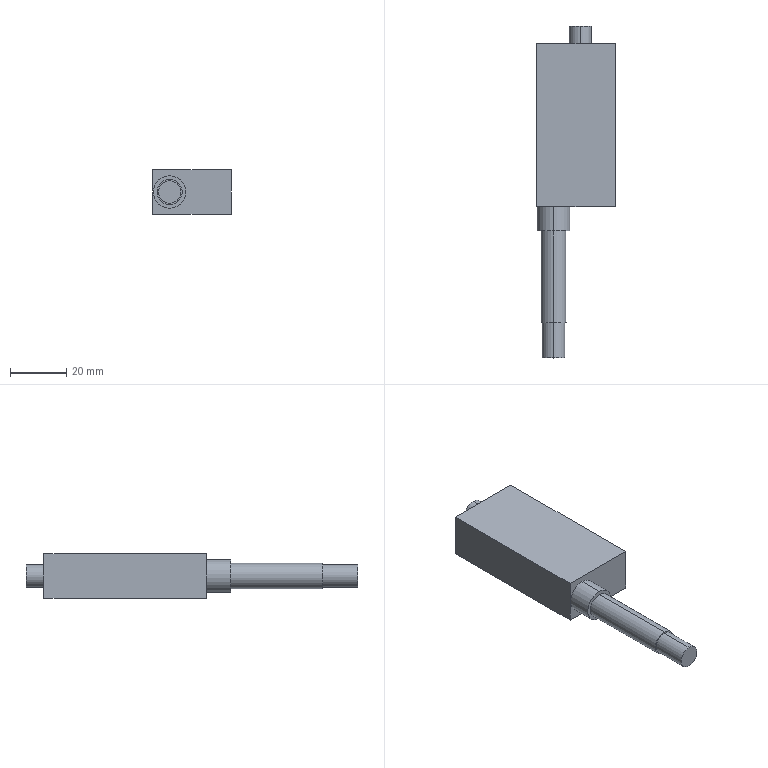Part | STEP file | Sensor head GT2-H12 | 1 solid | 18 faces | box 28 x 118.4 x 16 mm | volume 29940 mm3 | plane 10 | cylinder 8 | commonest cylinder face diameters 8 x4 9 x2 11.6 x2
STEP:
#1=CARTESIAN_POINT('',(0.,0.,0.));
#2=DIRECTION('',(0.,0.,1.));
#3=DIRECTION('',(1.,0.,0.));
#4=AXIS2_PLACEMENT_3D('',#1,#2,#3);
#5=CARTESIAN_POINT('',(-8.,-37.7,5.8));
#6=VERTEX_POINT('',#5);
#7=CARTESIAN_POINT('',(-8.,-37.7,-5.8));
#8=VERTEX_POINT('',#7);
#9=CARTESIAN_POINT('',(-8.,-37.7,0.));
#10=DIRECTION('',(0.,1.,0.));
#11=DIRECTION('',(0.,0.,1.));
#12=AXIS2_PLACEMENT_3D('',#9,#10,#11);
#13=CIRCLE('',#12,5.8);
#14=CARTESIAN_POINT('',(-8.,-37.7,0.));
#15=DIRECTION('',(0.,1.,0.));
#16=DIRECTION('',(0.,0.,1.));
#17=AXIS2_PLACEMENT_3D('',#14,#15,#16);
#18=CYLINDRICAL_SURFACE('',#17,5.8);
#19=CARTESIAN_POINT('',(0.,0.));
#20=DIRECTION('',(1.,0.));
#21=VECTOR('',#20,1.);
#22=LINE('',#19,#21);
#23=(GEOMETRIC_REPRESENTATION_CONTEXT(2)PARAMETRIC_REPRESENTATION_CONTEXT()REPRESENTATION_CONTEXT('',''));
#24=DEFINITIONAL_REPRESENTATION('',(#22),#23);
#25=PCURVE('',#18,#24);
#26=CARTESIAN_POINT('',(-8.,-37.7,0.));
#27=DIRECTION('',(0.,-1.,0.));
#28=DIRECTION('',(0.,0.,-1.));
#29=AXIS2_PLACEMENT_3D('',#26,#27,#28);
#30=PLANE('',#29);
#31=CARTESIAN_POINT('',(-5.8,0.));
#32=CARTESIAN_POINT('',(-5.8,10.046));
#33=CARTESIAN_POINT('',(2.9,5.023));
#34=CARTESIAN_POINT('',(11.6,0.));
#35=CARTESIAN_POINT('',(2.9,-5.023));
#36=CARTESIAN_POINT('',(-5.8,-10.046));
#37=CARTESIAN_POINT('',(-5.8,0.));
#38=(BOUNDED_CURVE()B_SPLINE_CURVE(2,(#31,#32,#33,#34,#35,#36,#37),.UNSPECIFIED.,.T.,.F.)B_SPLINE_CURVE_WITH_KNOTS((1,2,2,2,2,1),(-2.094,0.,2.094,4.189,6.283,8.378),.UNSPECIFIED.)CURVE()GEOMETRIC_REPRESENTATION_ITEM()RATIONAL_B_SPLINE_CURVE((1.,0.5,1.,0.5,1.,0.5,1.))REPRESENTATION_ITEM(''));
#39=(GEOMETRIC_REPRESENTATION_CONTEXT(2)PARAMETRIC_REPRESENTATION_CONTEXT()REPRESENTATION_CONTEXT('',''));
#40=DEFINITIONAL_REPRESENTATION('',(#38),#39);
#41=PCURVE('',#30,#40);
#42=SURFACE_CURVE('',#13,(#25,#41),.PCURVE_S1.);
#43=EDGE_CURVE('',#6,#8,#42,.T.);
#44=ORIENTED_EDGE('',*,*,#43,.T.);
#45=CARTESIAN_POINT('',(-8.,-29.,-5.8));
#46=VERTEX_POINT('',#45);
#47=CARTESIAN_POINT('',(-8.,-37.7,-5.8));
#48=DIRECTION('',(0.,1.,0.));
#49=VECTOR('',#48,1.);
#50=LINE('',#47,#49);
#51=CARTESIAN_POINT('',(3.142,0.));
#52=DIRECTION('',(0.,1.));
#53=VECTOR('',#52,1.);
#54=LINE('',#51,#53);
#55=(GEOMETRIC_REPRESENTATION_CONTEXT(2)PARAMETRIC_REPRESENTATION_CONTEXT()REPRESENTATION_CONTEXT('',''));
#56=DEFINITIONAL_REPRESENTATION('',(#54),#55);
#57=PCURVE('',#18,#56);
#58=CARTESIAN_POINT('',(-8.,-37.7,0.));
#59=DIRECTION('',(0.,1.,0.));
#60=DIRECTION('',(0.,0.,1.));
#61=AXIS2_PLACEMENT_3D('',#58,#59,#60);
#62=CYLINDRICAL_SURFACE('',#61,5.8);
#63=CARTESIAN_POINT('',(3.142,0.));
#64=DIRECTION('',(0.,1.));
#65=VECTOR('',#64,1.);
#66=LINE('',#63,#65);
#67=(GEOMETRIC_REPRESENTATION_CONTEXT(2)PARAMETRIC_REPRESENTATION_CONTEXT()REPRESENTATION_CONTEXT('',''));
#68=DEFINITIONAL_REPRESENTATION('',(#66),#67);
#69=PCURVE('',#62,#68);
#70=SURFACE_CURVE('',#50,(#57,#69),.PCURVE_S1.);
#71=EDGE_CURVE('',#8,#46,#70,.T.);
#72=ORIENTED_EDGE('',*,*,#71,.T.);
#73=CARTESIAN_POINT('',(-8.,-29.,5.8));
#74=VERTEX_POINT('',#73);
#75=CARTESIAN_POINT('',(-8.,-29.,0.));
#76=DIRECTION('',(0.,-1.,0.));
#77=DIRECTION('',(0.,0.,1.));
#78=AXIS2_PLACEMENT_3D('',#75,#76,#77);
#79=CIRCLE('',#78,5.8);
#80=CARTESIAN_POINT('',(6.283,8.7));
#81=DIRECTION('',(-1.,0.));
#82=VECTOR('',#81,1.);
#83=LINE('',#80,#82);
#84=(GEOMETRIC_REPRESENTATION_CONTEXT(2)PARAMETRIC_REPRESENTATION_CONTEXT()REPRESENTATION_CONTEXT('',''));
#85=DEFINITIONAL_REPRESENTATION('',(#83),#84);
#86=PCURVE('',#18,#85);
#87=CARTESIAN_POINT('',(-14.,-29.,8.));
#88=DIRECTION('',(0.,1.,0.));
#89=DIRECTION('',(0.,0.,1.));
#90=AXIS2_PLACEMENT_3D('',#87,#88,#89);
#91=PLANE('',#90);
#92=CARTESIAN_POINT('',(-2.2,6.));
#93=CARTESIAN_POINT('',(-2.2,-4.046));
#94=CARTESIAN_POINT('',(-10.9,0.9771));
#95=CARTESIAN_POINT('',(-19.6,6.));
#96=CARTESIAN_POINT('',(-10.9,11.023));
#97=CARTESIAN_POINT('',(-2.2,16.046));
#98=CARTESIAN_POINT('',(-2.2,6.));
#99=(BOUNDED_CURVE()B_SPLINE_CURVE(2,(#92,#93,#94,#95,#96,#97,#98),.UNSPECIFIED.,.T.,.F.)B_SPLINE_CURVE_WITH_KNOTS((1,2,2,2,2,1),(-2.094,0.,2.094,4.189,6.283,8.378),.UNSPECIFIED.)CURVE()GEOMETRIC_REPRESENTATION_ITEM()RATIONAL_B_SPLINE_CURVE((1.,0.5,1.,0.5,1.,0.5,1.))REPRESENTATION_ITEM(''));
#100=(GEOMETRIC_REPRESENTATION_CONTEXT(2)PARAMETRIC_REPRESENTATION_CONTEXT()REPRESENTATION_CONTEXT('',''));
#101=DEFINITIONAL_REPRESENTATION('',(#99),#100);
#102=PCURVE('',#91,#101);
#103=SURFACE_CURVE('',#79,(#86,#102),.PCURVE_S1.);
#104=EDGE_CURVE('',#46,#74,#103,.T.);
#105=ORIENTED_EDGE('',*,*,#104,.T.);
#106=CARTESIAN_POINT('',(-8.,-37.7,5.8));
#107=DIRECTION('',(0.,1.,0.));
#108=VECTOR('',#107,1.);
#109=LINE('',#106,#108);
#110=CARTESIAN_POINT('',(0.,0.));
#111=DIRECTION('',(0.,1.));
#112=VECTOR('',#111,1.);
#113=LINE('',#110,#112);
#114=(GEOMETRIC_REPRESENTATION_CONTEXT(2)PARAMETRIC_REPRESENTATION_CONTEXT()REPRESENTATION_CONTEXT('',''));
#115=DEFINITIONAL_REPRESENTATION('',(#113),#114);
#116=PCURVE('',#18,#115);
#117=CARTESIAN_POINT('',(6.283,0.));
#118=DIRECTION('',(0.,1.));
#119=VECTOR('',#118,1.);
#120=LINE('',#117,#119);
#121=(GEOMETRIC_REPRESENTATION_CONTEXT(2)PARAMETRIC_REPRESENTATION_CONTEXT()REPRESENTATION_CONTEXT('',''));
#122=DEFINITIONAL_REPRESENTATION('',(#120),#121);
#123=PCURVE('',#62,#122);
#124=SURFACE_CURVE('',#109,(#116,#123),.PCURVE_S1.);
#125=EDGE_CURVE('',#6,#74,#124,.T.);
#126=ORIENTED_EDGE('',*,*,#125,.F.);
#127=EDGE_LOOP('',(#44,#72,#105,#126));
#128=FACE_BOUND('',#127,.T.);
#129=ADVANCED_FACE('',(#128),#18,.T.);
#130=CARTESIAN_POINT('',(1.5,35.4,-4.));
#131=VERTEX_POINT('',#130);
#132=CARTESIAN_POINT('',(1.5,35.4,4.));
#133=VERTEX_POINT('',#132);
#134=CARTESIAN_POINT('',(1.5,35.4,0.));
#135=DIRECTION('',(0.,-1.,0.));
#136=DIRECTION('',(0.,0.,-1.));
#137=AXIS2_PLACEMENT_3D('',#134,#135,#136);
#138=CIRCLE('',#137,4.);
#139=CARTESIAN_POINT('',(1.5,35.4,0.));
#140=DIRECTION('',(0.,-1.,0.));
#141=DIRECTION('',(0.,0.,-1.));
#142=AXIS2_PLACEMENT_3D('',#139,#140,#141);
#143=CYLINDRICAL_SURFACE('',#142,4.);
#144=CARTESIAN_POINT('',(0.,0.));
#145=DIRECTION('',(1.,0.));
#146=VECTOR('',#145,1.);
#147=LINE('',#144,#146);
#148=(GEOMETRIC_REPRESENTATION_CONTEXT(2)PARAMETRIC_REPRESENTATION_CONTEXT()REPRESENTATION_CONTEXT('',''));
#149=DEFINITIONAL_REPRESENTATION('',(#147),#148);
#150=PCURVE('',#143,#149);
#151=CARTESIAN_POINT('',(1.5,35.4,0.));
#152=DIRECTION('',(0.,1.,0.));
#153=DIRECTION('',(0.,0.,1.));
#154=AXIS2_PLACEMENT_3D('',#151,#152,#153);
#155=PLANE('',#154);
#156=CARTESIAN_POINT('',(-4.,0.));
#157=CARTESIAN_POINT('',(-4.,6.928));
#158=CARTESIAN_POINT('',(2.,3.464));
#159=CARTESIAN_POINT('',(8.,0.));
#160=CARTESIAN_POINT('',(2.,-3.464));
#161=CARTESIAN_POINT('',(-4.,-6.928));
#162=CARTESIAN_POINT('',(-4.,0.));
#163=(BOUNDED_CURVE()B_SPLINE_CURVE(2,(#156,#157,#158,#159,#160,#161,#162),.UNSPECIFIED.,.T.,.F.)B_SPLINE_CURVE_WITH_KNOTS((1,2,2,2,2,1),(-2.094,0.,2.094,4.189,6.283,8.378),.UNSPECIFIED.)CURVE()GEOMETRIC_REPRESENTATION_ITEM()RATIONAL_B_SPLINE_CURVE((1.,0.5,1.,0.5,1.,0.5,1.))REPRESENTATION_ITEM(''));
#164=(GEOMETRIC_REPRESENTATION_CONTEXT(2)PARAMETRIC_REPRESENTATION_CONTEXT()REPRESENTATION_CONTEXT('',''));
#165=DEFINITIONAL_REPRESENTATION('',(#163),#164);
#166=PCURVE('',#155,#165);
#167=SURFACE_CURVE('',#138,(#150,#166),.PCURVE_S1.);
#168=EDGE_CURVE('',#131,#133,#167,.T.);
#169=ORIENTED_EDGE('',*,*,#168,.T.);
#170=CARTESIAN_POINT('',(1.5,29.,4.));
#171=VERTEX_POINT('',#170);
#172=CARTESIAN_POINT('',(1.5,35.4,4.));
#173=DIRECTION('',(0.,-1.,0.));
#174=VECTOR('',#173,1.);
#175=LINE('',#172,#174);
#176=CARTESIAN_POINT('',(3.142,0.));
#177=DIRECTION('',(0.,1.));
#178=VECTOR('',#177,1.);
#179=LINE('',#176,#178);
#180=(GEOMETRIC_REPRESENTATION_CONTEXT(2)PARAMETRIC_REPRESENTATION_CONTEXT()REPRESENTATION_CONTEXT('',''));
#181=DEFINITIONAL_REPRESENTATION('',(#179),#180);
#182=PCURVE('',#143,#181);
#183=CARTESIAN_POINT('',(1.5,35.4,0.));
#184=DIRECTION('',(0.,-1.,0.));
#185=DIRECTION('',(0.,0.,-1.));
#186=AXIS2_PLACEMENT_3D('',#183,#184,#185);
#187=CYLINDRICAL_SURFACE('',#186,4.);
#188=CARTESIAN_POINT('',(3.142,0.));
#189=DIRECTION('',(0.,1.));
#190=VECTOR('',#189,1.);
#191=LINE('',#188,#190);
#192=(GEOMETRIC_REPRESENTATION_CONTEXT(2)PARAMETRIC_REPRESENTATION_CONTEXT()REPRESENTATION_CONTEXT('',''));
#193=DEFINITIONAL_REPRESENTATION('',(#191),#192);
#194=PCURVE('',#187,#193);
#195=SURFACE_CURVE('',#175,(#182,#194),.PCURVE_S1.);
#196=EDGE_CURVE('',#133,#171,#195,.T.);
#197=ORIENTED_EDGE('',*,*,#196,.T.);
#198=CARTESIAN_POINT('',(1.5,29.,-4.));
#199=VERTEX_POINT('',#198);
#200=CARTESIAN_POINT('',(1.5,29.,0.));
#201=DIRECTION('',(0.,1.,0.));
#202=DIRECTION('',(0.,0.,-1.));
#203=AXIS2_PLACEMENT_3D('',#200,#201,#202);
#204=CIRCLE('',#203,4.);
#205=CARTESIAN_POINT('',(6.283,6.4));
#206=DIRECTION('',(-1.,0.));
#207=VECTOR('',#206,1.);
#208=LINE('',#205,#207);
#209=(GEOMETRIC_REPRESENTATION_CONTEXT(2)PARAMETRIC_REPRESENTATION_CONTEXT()REPRESENTATION_CONTEXT('',''));
#210=DEFINITIONAL_REPRESENTATION('',(#208),#209);
#211=PCURVE('',#143,#210);
#212=CARTESIAN_POINT('',(-14.,29.,8.));
#213=DIRECTION('',(0.,-1.,0.));
#214=DIRECTION('',(0.,0.,-1.));
#215=AXIS2_PLACEMENT_3D('',#212,#213,#214);
#216=PLANE('',#215);
#217=CARTESIAN_POINT('',(12.,15.5));
#218=CARTESIAN_POINT('',(12.,8.572));
#219=CARTESIAN_POINT('',(6.,12.036));
#220=CARTESIAN_POINT('',(0.,15.5));
#221=CARTESIAN_POINT('',(6.,18.964));
#222=CARTESIAN_POINT('',(12.,22.428));
#223=CARTESIAN_POINT('',(12.,15.5));
#224=(BOUNDED_CURVE()B_SPLINE_CURVE(2,(#217,#218,#219,#220,#221,#222,#223),.UNSPECIFIED.,.T.,.F.)B_SPLINE_CURVE_WITH_KNOTS((1,2,2,2,2,1),(-2.094,0.,2.094,4.189,6.283,8.378),.UNSPECIFIED.)CURVE()GEOMETRIC_REPRESENTATION_ITEM()RATIONAL_B_SPLINE_CURVE((1.,0.5,1.,0.5,1.,0.5,1.))REPRESENTATION_ITEM(''));
#225=(GEOMETRIC_REPRESENTATION_CONTEXT(2)PARAMETRIC_REPRESENTATION_CONTEXT()REPRESENTATION_CONTEXT('',''));
#226=DEFINITIONAL_REPRESENTATION('',(#224),#225);
#227=PCURVE('',#216,#226);
#228=SURFACE_CURVE('',#204,(#211,#227),.PCURVE_S1.);
#229=EDGE_CURVE('',#171,#199,#228,.T.);
#230=ORIENTED_EDGE('',*,*,#229,.T.);
#231=CARTESIAN_POINT('',(1.5,35.4,-4.));
#232=DIRECTION('',(0.,-1.,0.));
#233=VECTOR('',#232,1.);
#234=LINE('',#231,#233);
#235=CARTESIAN_POINT('',(0.,0.));
#236=DIRECTION('',(0.,1.));
#237=VECTOR('',#236,1.);
#238=LINE('',#235,#237);
#239=(GEOMETRIC_REPRESENTATION_CONTEXT(2)PARAMETRIC_REPRESENTATION_CONTEXT()REPRESENTATION_CONTEXT('',''));
#240=DEFINITIONAL_REPRESENTATION('',(#238),#239);
#241=PCURVE('',#143,#240);
#242=CARTESIAN_POINT('',(6.283,0.));
#243=DIRECTION('',(0.,1.));
#244=VECTOR('',#243,1.);
#245=LINE('',#242,#244);
#246=(GEOMETRIC_REPRESENTATION_CONTEXT(2)PARAMETRIC_REPRESENTATION_CONTEXT()REPRESENTATION_CONTEXT('',''));
#247=DEFINITIONAL_REPRESENTATION('',(#245),#246);
#248=PCURVE('',#187,#247);
#249=SURFACE_CURVE('',#234,(#241,#248),.PCURVE_S1.);
#250=EDGE_CURVE('',#131,#199,#249,.T.);
#251=ORIENTED_EDGE('',*,*,#250,.F.);
#252=EDGE_LOOP('',(#169,#197,#230,#251));
#253=FACE_BOUND('',#252,.T.);
#254=ADVANCED_FACE('',(#253),#143,.T.);
#255=CARTESIAN_POINT('',(-8.,-70.5,4.5));
#256=VERTEX_POINT('',#255);
#257=CARTESIAN_POINT('',(-8.,-70.5,-4.5));
#258=VERTEX_POINT('',#257);
#259=CARTESIAN_POINT('',(-8.,-70.5,0.));
#260=DIRECTION('',(0.,1.,0.));
#261=DIRECTION('',(0.,0.,1.));
#262=AXIS2_PLACEMENT_3D('',#259,#260,#261);
#263=CIRCLE('',#262,4.5);
#264=CARTESIAN_POINT('',(-8.,-70.5,0.));
#265=DIRECTION('',(0.,1.,0.));
#266=DIRECTION('',(0.,0.,1.));
#267=AXIS2_PLACEMENT_3D('',#264,#265,#266);
#268=CYLINDRICAL_SURFACE('',#267,4.5);
#269=CARTESIAN_POINT('',(0.,0.));
#270=DIRECTION('',(1.,0.));
#271=VECTOR('',#270,1.);
#272=LINE('',#269,#271);
#273=(GEOMETRIC_REPRESENTATION_CONTEXT(2)PARAMETRIC_REPRESENTATION_CONTEXT()REPRESENTATION_CONTEXT('',''));
#274=DEFINITIONAL_REPRESENTATION('',(#272),#273);
#275=PCURVE('',#268,#274);
#276=CARTESIAN_POINT('',(-8.,-70.5,0.));
#277=DIRECTION('',(0.,-1.,0.));
#278=DIRECTION('',(0.,0.,-1.));
#279=AXIS2_PLACEMENT_3D('',#276,#277,#278);
#280=PLANE('',#279);
#281=CARTESIAN_POINT('',(-4.5,0.));
#282=CARTESIAN_POINT('',(-4.5,7.794));
#283=CARTESIAN_POINT('',(2.25,3.897));
#284=CARTESIAN_POINT('',(9.,0.));
#285=CARTESIAN_POINT('',(2.25,-3.897));
#286=CARTESIAN_POINT('',(-4.5,-7.794));
#287=CARTESIAN_POINT('',(-4.5,0.));
#288=(BOUNDED_CURVE()B_SPLINE_CURVE(2,(#281,#282,#283,#284,#285,#286,#287),.UNSPECIFIED.,.T.,.F.)B_SPLINE_CURVE_WITH_KNOTS((1,2,2,2,2,1),(-2.094,0.,2.094,4.189,6.283,8.378),.UNSPECIFIED.)CURVE()GEOMETRIC_REPRESENTATION_ITEM()RATIONAL_B_SPLINE_CURVE((1.,0.5,1.,0.5,1.,0.5,1.))REPRESENTATION_ITEM(''));
#289=(GEOMETRIC_REPRESENTATION_CONTEXT(2)PARAMETRIC_REPRESENTATION_CONTEXT()REPRESENTATION_CONTEXT('',''));
#290=DEFINITIONAL_REPRESENTATION('',(#288),#289);
#291=PCURVE('',#280,#290);
#292=SURFACE_CURVE('',#263,(#275,#291),.PCURVE_S1.);
#293=EDGE_CURVE('',#256,#258,#292,.T.);
#294=ORIENTED_EDGE('',*,*,#293,.T.);
#295=CARTESIAN_POINT('',(-8.,-37.7,-4.5));
#296=VERTEX_POINT('',#295);
#297=CARTESIAN_POINT('',(-8.,-70.5,-4.5));
#298=DIRECTION('',(0.,1.,0.));
#299=VECTOR('',#298,1.);
#300=LINE('',#297,#299);
#301=CARTESIAN_POINT('',(3.142,0.));
#302=DIRECTION('',(0.,1.));
#303=VECTOR('',#302,1.);
#304=LINE('',#301,#303);
#305=(GEOMETRIC_REPRESENTATION_CONTEXT(2)PARAMETRIC_REPRESENTATION_CONTEXT()REPRESENTATION_CONTEXT('',''));
#306=DEFINITIONAL_REPRESENTATION('',(#304),#305);
#307=PCURVE('',#268,#306);
#308=CARTESIAN_POINT('',(-8.,-70.5,0.));
#309=DIRECTION('',(0.,1.,0.));
#310=DIRECTION('',(0.,0.,1.));
#311=AXIS2_PLACEMENT_3D('',#308,#309,#310);
#312=CYLINDRICAL_SURFACE('',#311,4.5);
#313=CARTESIAN_POINT('',(3.142,0.));
#314=DIRECTION('',(0.,1.));
#315=VECTOR('',#314,1.);
#316=LINE('',#313,#315);
#317=(GEOMETRIC_REPRESENTATION_CONTEXT(2)PARAMETRIC_REPRESENTATION_CONTEXT()REPRESENTATION_CONTEXT('',''));
#318=DEFINITIONAL_REPRESENTATION('',(#316),#317);
#319=PCURVE('',#312,#318);
#320=SURFACE_CURVE('',#300,(#307,#319),.PCURVE_S1.);
#321=EDGE_CURVE('',#258,#296,#320,.T.);
#322=ORIENTED_EDGE('',*,*,#321,.T.);
#323=CARTESIAN_POINT('',(-8.,-37.7,4.5));
#324=VERTEX_POINT('',#323);
#325=CARTESIAN_POINT('',(-8.,-37.7,0.));
#326=DIRECTION('',(0.,1.,0.));
#327=DIRECTION('',(0.,0.,1.));
#328=AXIS2_PLACEMENT_3D('',#325,#326,#327);
#329=CIRCLE('',#328,4.5);
#330=CARTESIAN_POINT('',(0.,32.8));
#331=DIRECTION('',(1.,0.));
#332=VECTOR('',#331,1.);
#333=LINE('',#330,#332);
#334=(GEOMETRIC_REPRESENTATION_CONTEXT(2)PARAMETRIC_REPRESENTATION_CONTEXT()REPRESENTATION_CONTEXT('',''));
#335=DEFINITIONAL_REPRESENTATION('',(#333),#334);
#336=PCURVE('',#268,#335);
#337=CARTESIAN_POINT('',(-4.5,0.));
#338=CARTESIAN_POINT('',(-4.5,7.794));
#339=CARTESIAN_POINT('',(2.25,3.897));
#340=CARTESIAN_POINT('',(9.,0.));
#341=CARTESIAN_POINT('',(2.25,-3.897));
#342=CARTESIAN_POINT('',(-4.5,-7.794));
#343=CARTESIAN_POINT('',(-4.5,0.));
#344=(BOUNDED_CURVE()B_SPLINE_CURVE(2,(#337,#338,#339,#340,#341,#342,#343),.UNSPECIFIED.,.T.,.F.)B_SPLINE_CURVE_WITH_KNOTS((1,2,2,2,2,1),(-2.094,0.,2.094,4.189,6.283,8.378),.UNSPECIFIED.)CURVE()GEOMETRIC_REPRESENTATION_ITEM()RATIONAL_B_SPLINE_CURVE((1.,0.5,1.,0.5,1.,0.5,1.))REPRESENTATION_ITEM(''));
#345=(GEOMETRIC_REPRESENTATION_CONTEXT(2)PARAMETRIC_REPRESENTATION_CONTEXT()REPRESENTATION_CONTEXT('',''));
#346=DEFINITIONAL_REPRESENTATION('',(#344),#345);
#347=PCURVE('',#30,#346);
#348=SURFACE_CURVE('',#329,(#336,#347),.PCURVE_S1.);
#349=EDGE_CURVE('',#324,#296,#348,.T.);
#350=ORIENTED_EDGE('',*,*,#349,.F.);
#351=CARTESIAN_POINT('',(-8.,-70.5,4.5));
#352=DIRECTION('',(0.,1.,0.));
#353=VECTOR('',#352,1.);
#354=LINE('',#351,#353);
#355=CARTESIAN_POINT('',(0.,0.));
#356=DIRECTION('',(0.,1.));
#357=VECTOR('',#356,1.);
#358=LINE('',#355,#357);
#359=(GEOMETRIC_REPRESENTATION_CONTEXT(2)PARAMETRIC_REPRESENTATION_CONTEXT()REPRESENTATION_CONTEXT('',''));
#360=DEFINITIONAL_REPRESENTATION('',(#358),#359);
#361=PCURVE('',#268,#360);
#362=CARTESIAN_POINT('',(6.283,0.));
#363=DIRECTION('',(0.,1.));
#364=VECTOR('',#363,1.);
#365=LINE('',#362,#364);
#366=(GEOMETRIC_REPRESENTATION_CONTEXT(2)PARAMETRIC_REPRESENTATION_CONTEXT()REPRESENTATION_CONTEXT('',''));
#367=DEFINITIONAL_REPRESENTATION('',(#365),#366);
#368=PCURVE('',#312,#367);
#369=SURFACE_CURVE('',#354,(#361,#368),.PCURVE_S1.);
#370=EDGE_CURVE('',#256,#324,#369,.T.);
#371=ORIENTED_EDGE('',*,*,#370,.F.);
#372=EDGE_LOOP('',(#294,#322,#350,#371));
#373=FACE_BOUND('',#372,.T.);
#374=ADVANCED_FACE('',(#373),#268,.T.);
#375=CARTESIAN_POINT('',(-8.,-83.,4.));
#376=VERTEX_POINT('',#375);
#377=CARTESIAN_POINT('',(-8.,-83.,-4.));
#378=VERTEX_POINT('',#377);
#379=CARTESIAN_POINT('',(-8.,-83.,0.));
#380=DIRECTION('',(0.,1.,0.));
#381=DIRECTION('',(0.,0.,1.));
#382=AXIS2_PLACEMENT_3D('',#379,#380,#381);
#383=CIRCLE('',#382,4.);
#384=CARTESIAN_POINT('',(-8.,-83.,0.));
#385=DIRECTION('',(0.,1.,0.));
#386=DIRECTION('',(0.,0.,1.));
#387=AXIS2_PLACEMENT_3D('',#384,#385,#386);
#388=CYLINDRICAL_SURFACE('',#387,4.);
#389=CARTESIAN_POINT('',(0.,0.));
#390=DIRECTION('',(1.,0.));
#391=VECTOR('',#390,1.);
#392=LINE('',#389,#391);
#393=(GEOMETRIC_REPRESENTATION_CONTEXT(2)PARAMETRIC_REPRESENTATION_CONTEXT()REPRESENTATION_CONTEXT('',''));
#394=DEFINITIONAL_REPRESENTATION('',(#392),#393);
#395=PCURVE('',#388,#394);
#396=CARTESIAN_POINT('',(-8.,-83.,0.));
#397=DIRECTION('',(0.,-1.,0.));
#398=DIRECTION('',(0.,0.,-1.));
#399=AXIS2_PLACEMENT_3D('',#396,#397,#398);
#400=PLANE('',#399);
#401=CARTESIAN_POINT('',(-4.,0.));
#402=CARTESIAN_POINT('',(-4.,6.928));
#403=CARTESIAN_POINT('',(2.,3.464));
#404=CARTESIAN_POINT('',(8.,0.));
#405=CARTESIAN_POINT('',(2.,-3.464));
#406=CARTESIAN_POINT('',(-4.,-6.928));
#407=CARTESIAN_POINT('',(-4.,0.));
#408=(BOUNDED_CURVE()B_SPLINE_CURVE(2,(#401,#402,#403,#404,#405,#406,#407),.UNSPECIFIED.,.T.,.F.)B_SPLINE_CURVE_WITH_KNOTS((1,2,2,2,2,1),(-2.094,0.,2.094,4.189,6.283,8.378),.UNSPECIFIED.)CURVE()GEOMETRIC_REPRESENTATION_ITEM()RATIONAL_B_SPLINE_CURVE((1.,0.5,1.,0.5,1.,0.5,1.))REPRESENTATION_ITEM(''));
#409=(GEOMETRIC_REPRESENTATION_CONTEXT(2)PARAMETRIC_REPRESENTATION_CONTEXT()REPRESENTATION_CONTEXT('',''));
#410=DEFINITIONAL_REPRESENTATION('',(#408),#409);
#411=PCURVE('',#400,#410);
#412=SURFACE_CURVE('',#383,(#395,#411),.PCURVE_S1.);
#413=EDGE_CURVE('',#376,#378,#412,.T.);
#414=ORIENTED_EDGE('',*,*,#413,.T.);
#415=CARTESIAN_POINT('',(-8.,-70.5,-4.));
#416=VERTEX_POINT('',#415);
#417=CARTESIAN_POINT('',(-8.,-83.,-4.));
#418=DIRECTION('',(0.,1.,0.));
#419=VECTOR('',#418,1.);
#420=LINE('',#417,#419);
#421=CARTESIAN_POINT('',(3.142,0.));
#422=DIRECTION('',(0.,1.));
#423=VECTOR('',#422,1.);
#424=LINE('',#421,#423);
#425=(GEOMETRIC_REPRESENTATION_CONTEXT(2)PARAMETRIC_REPRESENTATION_CONTEXT()REPRESENTATION_CONTEXT('',''));
#426=DEFINITIONAL_REPRESENTATION('',(#424),#425);
#427=PCURVE('',#388,#426);
#428=CARTESIAN_POINT('',(-8.,-83.,0.));
#429=DIRECTION('',(0.,1.,0.));
#430=DIRECTION('',(0.,0.,1.));
#431=AXIS2_PLACEMENT_3D('',#428,#429,#430);
#432=CYLINDRICAL_SURFACE('',#431,4.);
#433=CARTESIAN_POINT('',(3.142,0.));
#434=DIRECTION('',(0.,1.));
#435=VECTOR('',#434,1.);
#436=LINE('',#433,#435);
#437=(GEOMETRIC_REPRESENTATION_CONTEXT(2)PARAMETRIC_REPRESENTATION_CONTEXT()REPRESENTATION_CONTEXT('',''));
#438=DEFINITIONAL_REPRESENTATION('',(#436),#437);
#439=PCURVE('',#432,#438);
#440=SURFACE_CURVE('',#420,(#427,#439),.PCURVE_S1.);
#441=EDGE_CURVE('',#378,#416,#440,.T.);
#442=ORIENTED_EDGE('',*,*,#441,.T.);
#443=CARTESIAN_POINT('',(-8.,-70.5,4.));
#444=VERTEX_POINT('',#443);
#445=CARTESIAN_POINT('',(-8.,-70.5,0.));
#446=DIRECTION('',(0.,1.,0.));
#447=DIRECTION('',(0.,0.,1.));
#448=AXIS2_PLACEMENT_3D('',#445,#446,#447);
#449=CIRCLE('',#448,4.);
#450=CARTESIAN_POINT('',(0.,12.5));
#451=DIRECTION('',(1.,0.));
#452=VECTOR('',#451,1.);
#453=LINE('',#450,#452);
#454=(GEOMETRIC_REPRESENTATION_CONTEXT(2)PARAMETRIC_REPRESENTATION_CONTEXT()REPRESENTATION_CONTEXT('',''));
#455=DEFINITIONAL_REPRESENTATION('',(#453),#454);
#456=PCURVE('',#388,#455);
#457=CARTESIAN_POINT('',(-4.,0.));
#458=CARTESIAN_POINT('',(-4.,6.928));
#459=CARTESIAN_POINT('',(2.,3.464));
#460=CARTESIAN_POINT('',(8.,0.));
#461=CARTESIAN_POINT('',(2.,-3.464));
#462=CARTESIAN_POINT('',(-4.,-6.928));
#463=CARTESIAN_POINT('',(-4.,0.));
#464=(BOUNDED_CURVE()B_SPLINE_CURVE(2,(#457,#458,#459,#460,#461,#462,#463),.UNSPECIFIED.,.T.,.F.)B_SPLINE_CURVE_WITH_KNOTS((1,2,2,2,2,1),(-2.094,0.,2.094,4.189,6.283,8.378),.UNSPECIFIED.)CURVE()GEOMETRIC_REPRESENTATION_ITEM()RATIONAL_B_SPLINE_CURVE((1.,0.5,1.,0.5,1.,0.5,1.))REPRESENTATION_ITEM(''));
#465=(GEOMETRIC_REPRESENTATION_CONTEXT(2)PARAMETRIC_REPRESENTATION_CONTEXT()REPRESENTATION_CONTEXT('',''));
#466=DEFINITIONAL_REPRESENTATION('',(#464),#465);
#467=PCURVE('',#280,#466);
#468=SURFACE_CURVE('',#449,(#456,#467),.PCURVE_S1.);
#469=EDGE_CURVE('',#444,#416,#468,.T.);
#470=ORIENTED_EDGE('',*,*,#469,.F.);
#471=CARTESIAN_POINT('',(-8.,-83.,4.));
#472=DIRECTION('',(0.,1.,0.));
#473=VECTOR('',#472,1.);
#474=LINE('',#471,#473);
#475=CARTESIAN_POINT('',(0.,0.));
#476=DIRECTION('',(0.,1.));
#477=VECTOR('',#476,1.);
#478=LINE('',#475,#477);
#479=(GEOMETRIC_REPRESENTATION_CONTEXT(2)PARAMETRIC_REPRESENTATION_CONTEXT()REPRESENTATION_CONTEXT('',''));
#480=DEFINITIONAL_REPRESENTATION('',(#478),#479);
#481=PCURVE('',#388,#480);
#482=CARTESIAN_POINT('',(6.283,0.));
#483=DIRECTION('',(0.,1.));
#484=VECTOR('',#483,1.);
#485=LINE('',#482,#484);
#486=(GEOMETRIC_REPRESENTATION_CONTEXT(2)PARAMETRIC_REPRESENTATION_CONTEXT()REPRESENTATION_CONTEXT('',''));
#487=DEFINITIONAL_REPRESENTATION('',(#485),#486);
#488=PCURVE('',#432,#487);
#489=SURFACE_CURVE('',#474,(#481,#488),.PCURVE_S1.);
#490=EDGE_CURVE('',#376,#444,#489,.T.);
#491=ORIENTED_EDGE('',*,*,#490,.F.);
#492=EDGE_LOOP('',(#414,#442,#470,#491));
#493=FACE_BOUND('',#492,.T.);
#494=ADVANCED_FACE('',(#493),#388,.T.);
#495=CARTESIAN_POINT('',(-14.,29.,8.));
#496=VERTEX_POINT('',#495);
#497=CARTESIAN_POINT('',(-14.,-29.,8.));
#498=VERTEX_POINT('',#497);
#499=CARTESIAN_POINT('',(-14.,-29.,8.));
#500=DIRECTION('',(0.,-1.,0.));
#501=VECTOR('',#500,1.);
#502=LINE('',#499,#501);
#503=CARTESIAN_POINT('',(14.,-29.,8.));
#504=DIRECTION('',(0.,0.,1.));
#505=DIRECTION('',(1.,0.,0.));
#506=AXIS2_PLACEMENT_3D('',#503,#504,#505);
#507=PLANE('',#506);
#508=CARTESIAN_POINT('',(-28.,0.));
#509=DIRECTION('',(0.,-1.));
#510=VECTOR('',#509,1.);
#511=LINE('',#508,#510);
#512=(GEOMETRIC_REPRESENTATION_CONTEXT(2)PARAMETRIC_REPRESENTATION_CONTEXT()REPRESENTATION_CONTEXT('',''));
#513=DEFINITIONAL_REPRESENTATION('',(#511),#512);
#514=PCURVE('',#507,#513);
#515=CARTESIAN_POINT('',(-14.,29.,8.));
#516=DIRECTION('',(1.,0.,0.));
#517=DIRECTION('',(0.,1.,0.));
#518=AXIS2_PLACEMENT_3D('',#515,#516,#517);
#519=PLANE('',#518);
#520=CARTESIAN_POINT('',(-58.,0.));
#521=DIRECTION('',(-1.,0.));
#522=VECTOR('',#521,1.);
#523=LINE('',#520,#522);
#524=(GEOMETRIC_REPRESENTATION_CONTEXT(2)PARAMETRIC_REPRESENTATION_CONTEXT()REPRESENTATION_CONTEXT('',''));
#525=DEFINITIONAL_REPRESENTATION('',(#523),#524);
#526=PCURVE('',#519,#525);
#527=SURFACE_CURVE('',#502,(#514,#526),.PCURVE_S1.);
#528=EDGE_CURVE('',#496,#498,#527,.T.);
#529=ORIENTED_EDGE('',*,*,#528,.T.);
#530=CARTESIAN_POINT('',(14.,-29.,8.));
#531=VERTEX_POINT('',#530);
#532=CARTESIAN_POINT('',(14.,-29.,8.));
#533=DIRECTION('',(1.,0.,0.));
#534=VECTOR('',#533,1.);
#535=LINE('',#532,#534);
#536=CARTESIAN_POINT('',(0.,0.));
#537=DIRECTION('',(1.,0.));
#538=VECTOR('',#537,1.);
#539=LINE('',#536,#538);
#540=(GEOMETRIC_REPRESENTATION_CONTEXT(2)PARAMETRIC_REPRESENTATION_CONTEXT()REPRESENTATION_CONTEXT('',''));
#541=DEFINITIONAL_REPRESENTATION('',(#539),#540);
#542=PCURVE('',#507,#541);
#543=CARTESIAN_POINT('',(0.,28.));
#544=DIRECTION('',(0.,1.));
#545=VECTOR('',#544,1.);
#546=LINE('',#543,#545);
#547=(GEOMETRIC_REPRESENTATION_CONTEXT(2)PARAMETRIC_REPRESENTATION_CONTEXT()REPRESENTATION_CONTEXT('',''));
#548=DEFINITIONAL_REPRESENTATION('',(#546),#547);
#549=PCURVE('',#91,#548);
#550=SURFACE_CURVE('',#535,(#542,#549),.PCURVE_S1.);
#551=EDGE_CURVE('',#498,#531,#550,.T.);
#552=ORIENTED_EDGE('',*,*,#551,.T.);
#553=CARTESIAN_POINT('',(14.,29.,8.));
#554=VERTEX_POINT('',#553);
#555=CARTESIAN_POINT('',(14.,-29.,8.));
#556=DIRECTION('',(0.,1.,0.));
#557=VECTOR('',#556,1.);
#558=LINE('',#555,#557);
#559=CARTESIAN_POINT('',(0.,0.));
#560=DIRECTION('',(0.,1.));
#561=VECTOR('',#560,1.);
#562=LINE('',#559,#561);
#563=(GEOMETRIC_REPRESENTATION_CONTEXT(2)PARAMETRIC_REPRESENTATION_CONTEXT()REPRESENTATION_CONTEXT('',''));
#564=DEFINITIONAL_REPRESENTATION('',(#562),#563);
#565=PCURVE('',#507,#564);
#566=CARTESIAN_POINT('',(14.,29.,8.));
#567=DIRECTION('',(-1.,0.,0.));
#568=DIRECTION('',(0.,-1.,0.));
#569=AXIS2_PLACEMENT_3D('',#566,#567,#568);
#570=PLANE('',#569);
#571=CARTESIAN_POINT('',(58.,0.));
#572=DIRECTION('',(-1.,0.));
#573=VECTOR('',#572,1.);
#574=LINE('',#571,#573);
#575=(GEOMETRIC_REPRESENTATION_CONTEXT(2)PARAMETRIC_REPRESENTATION_CONTEXT()REPRESENTATION_CONTEXT('',''));
#576=DEFINITIONAL_REPRESENTATION('',(#574),#575);
#577=PCURVE('',#570,#576);
#578=SURFACE_CURVE('',#558,(#565,#577),.PCURVE_S1.);
#579=EDGE_CURVE('',#531,#554,#578,.T.);
#580=ORIENTED_EDGE('',*,*,#579,.T.);
#581=CARTESIAN_POINT('',(14.,29.,8.));
#582=DIRECTION('',(-1.,0.,0.));
#583=VECTOR('',#582,1.);
#584=LINE('',#581,#583);
#585=CARTESIAN_POINT('',(0.,58.));
#586=DIRECTION('',(-1.,0.));
#587=VECTOR('',#586,1.);
#588=LINE('',#585,#587);
#589=(GEOMETRIC_REPRESENTATION_CONTEXT(2)PARAMETRIC_REPRESENTATION_CONTEXT()REPRESENTATION_CONTEXT('',''));
#590=DEFINITIONAL_REPRESENTATION('',(#588),#589);
#591=PCURVE('',#507,#590);
#592=CARTESIAN_POINT('',(0.,28.));
#593=DIRECTION('',(0.,-1.));
#594=VECTOR('',#593,1.);
#595=LINE('',#592,#594);
#596=(GEOMETRIC_REPRESENTATION_CONTEXT(2)PARAMETRIC_REPRESENTATION_CONTEXT()REPRESENTATION_CONTEXT('',''));
#597=DEFINITIONAL_REPRESENTATION('',(#595),#596);
#598=PCURVE('',#216,#597);
#599=SURFACE_CURVE('',#584,(#591,#598),.PCURVE_S1.);
#600=EDGE_CURVE('',#554,#496,#599,.T.);
#601=ORIENTED_EDGE('',*,*,#600,.T.);
#602=EDGE_LOOP('',(#529,#552,#580,#601));
#603=FACE_BOUND('',#602,.T.);
#604=ADVANCED_FACE('',(#603),#507,.T.);
#605=CARTESIAN_POINT('',(-8.,-29.,0.));
#606=DIRECTION('',(0.,-1.,0.));
#607=DIRECTION('',(0.,0.,1.));
#608=AXIS2_PLACEMENT_3D('',#605,#606,#607);
#609=CIRCLE('',#608,5.8);
#610=CARTESIAN_POINT('',(-2.2,6.));
#611=CARTESIAN_POINT('',(-2.2,-4.046));
#612=CARTESIAN_POINT('',(-10.9,0.9771));
#613=CARTESIAN_POINT('',(-19.6,6.));
#614=CARTESIAN_POINT('',(-10.9,11.023));
#615=CARTESIAN_POINT('',(-2.2,16.046));
#616=CARTESIAN_POINT('',(-2.2,6.));
#617=(BOUNDED_CURVE()B_SPLINE_CURVE(2,(#610,#611,#612,#613,#614,#615,#616),.UNSPECIFIED.,.T.,.F.)B_SPLINE_CURVE_WITH_KNOTS((1,2,2,2,2,1),(-2.094,0.,2.094,4.189,6.283,8.378),.UNSPECIFIED.)CURVE()GEOMETRIC_REPRESENTATION_ITEM()RATIONAL_B_SPLINE_CURVE((1.,0.5,1.,0.5,1.,0.5,1.))REPRESENTATION_ITEM(''));
#618=(GEOMETRIC_REPRESENTATION_CONTEXT(2)PARAMETRIC_REPRESENTATION_CONTEXT()REPRESENTATION_CONTEXT('',''));
#619=DEFINITIONAL_REPRESENTATION('',(#617),#618);
#620=PCURVE('',#91,#619);
#621=CARTESIAN_POINT('',(6.283,8.7));
#622=DIRECTION('',(-1.,0.));
#623=VECTOR('',#622,1.);
#624=LINE('',#621,#623);
#625=(GEOMETRIC_REPRESENTATION_CONTEXT(2)PARAMETRIC_REPRESENTATION_CONTEXT()REPRESENTATION_CONTEXT('',''));
#626=DEFINITIONAL_REPRESENTATION('',(#624),#625);
#627=PCURVE('',#62,#626);
#628=SURFACE_CURVE('',#609,(#620,#627),.PCURVE_S1.);
#629=EDGE_CURVE('',#74,#46,#628,.T.);
#630=ORIENTED_EDGE('',*,*,#629,.F.);
#631=ORIENTED_EDGE('',*,*,#104,.F.);
#632=EDGE_LOOP('',(#630,#631));
#633=FACE_BOUND('',#632,.T.);
#634=CARTESIAN_POINT('',(14.,-29.,-8.));
#635=VERTEX_POINT('',#634);
#636=CARTESIAN_POINT('',(14.,-29.,8.));
#637=DIRECTION('',(0.,0.,-1.));
#638=VECTOR('',#637,1.);
#639=LINE('',#636,#638);
#640=CARTESIAN_POINT('',(0.,28.));
#641=DIRECTION('',(-1.,0.));
#642=VECTOR('',#641,1.);
#643=LINE('',#640,#642);
#644=(GEOMETRIC_REPRESENTATION_CONTEXT(2)PARAMETRIC_REPRESENTATION_CONTEXT()REPRESENTATION_CONTEXT('',''));
#645=DEFINITIONAL_REPRESENTATION('',(#643),#644);
#646=PCURVE('',#91,#645);
#647=CARTESIAN_POINT('',(58.,0.));
#648=DIRECTION('',(0.,-1.));
#649=VECTOR('',#648,1.);
#650=LINE('',#647,#649);
#651=(GEOMETRIC_REPRESENTATION_CONTEXT(2)PARAMETRIC_REPRESENTATION_CONTEXT()REPRESENTATION_CONTEXT('',''));
#652=DEFINITIONAL_REPRESENTATION('',(#650),#651);
#653=PCURVE('',#570,#652);
#654=SURFACE_CURVE('',#639,(#646,#653),.PCURVE_S1.);
#655=EDGE_CURVE('',#531,#635,#654,.T.);
#656=ORIENTED_EDGE('',*,*,#655,.F.);
#657=ORIENTED_EDGE('',*,*,#551,.F.);
#658=CARTESIAN_POINT('',(-14.,-29.,-8.));
#659=VERTEX_POINT('',#658);
#660=CARTESIAN_POINT('',(-14.,-29.,8.));
#661=DIRECTION('',(0.,0.,1.));
#662=VECTOR('',#661,1.);
#663=LINE('',#660,#662);
#664=CARTESIAN_POINT('',(0.,0.));
#665=DIRECTION('',(1.,0.));
#666=VECTOR('',#665,1.);
#667=LINE('',#664,#666);
#668=(GEOMETRIC_REPRESENTATION_CONTEXT(2)PARAMETRIC_REPRESENTATION_CONTEXT()REPRESENTATION_CONTEXT('',''));
#669=DEFINITIONAL_REPRESENTATION('',(#667),#668);
#670=PCURVE('',#91,#669);
#671=CARTESIAN_POINT('',(-58.,0.));
#672=DIRECTION('',(0.,1.));
#673=VECTOR('',#672,1.);
#674=LINE('',#671,#673);
#675=(GEOMETRIC_REPRESENTATION_CONTEXT(2)PARAMETRIC_REPRESENTATION_CONTEXT()REPRESENTATION_CONTEXT('',''));
#676=DEFINITIONAL_REPRESENTATION('',(#674),#675);
#677=PCURVE('',#519,#676);
#678=SURFACE_CURVE('',#663,(#670,#677),.PCURVE_S1.);
#679=EDGE_CURVE('',#659,#498,#678,.T.);
#680=ORIENTED_EDGE('',*,*,#679,.F.);
#681=CARTESIAN_POINT('',(-14.,-29.,-8.));
#682=DIRECTION('',(-1.,0.,0.));
#683=VECTOR('',#682,1.);
#684=LINE('',#681,#683);
#685=CARTESIAN_POINT('',(-16.,0.));
#686=DIRECTION('',(0.,-1.));
#687=VECTOR('',#686,1.);
#688=LINE('',#685,#687);
#689=(GEOMETRIC_REPRESENTATION_CONTEXT(2)PARAMETRIC_REPRESENTATION_CONTEXT()REPRESENTATION_CONTEXT('',''));
#690=DEFINITIONAL_REPRESENTATION('',(#688),#689);
#691=PCURVE('',#91,#690);
#692=CARTESIAN_POINT('',(14.,-29.,-8.));
#693=DIRECTION('',(0.,0.,1.));
#694=DIRECTION('',(1.,0.,0.));
#695=AXIS2_PLACEMENT_3D('',#692,#693,#694);
#696=PLANE('',#695);
#697=CARTESIAN_POINT('',(-28.,0.));
#698=DIRECTION('',(-1.,0.));
#699=VECTOR('',#698,1.);
#700=LINE('',#697,#699);
#701=(GEOMETRIC_REPRESENTATION_CONTEXT(2)PARAMETRIC_REPRESENTATION_CONTEXT()REPRESENTATION_CONTEXT('',''));
#702=DEFINITIONAL_REPRESENTATION('',(#700),#701);
#703=PCURVE('',#696,#702);
#704=SURFACE_CURVE('',#684,(#691,#703),.PCURVE_S1.);
#705=EDGE_CURVE('',#635,#659,#704,.T.);
#706=ORIENTED_EDGE('',*,*,#705,.F.);
#707=EDGE_LOOP('',(#656,#657,#680,#706));
#708=FACE_BOUND('',#707,.T.);
#709=ADVANCED_FACE('',(#633,#708),#91,.F.);
#710=ORIENTED_EDGE('',*,*,#679,.T.);
#711=ORIENTED_EDGE('',*,*,#528,.F.);
#712=CARTESIAN_POINT('',(-14.,29.,-8.));
#713=VERTEX_POINT('',#712);
#714=CARTESIAN_POINT('',(-14.,29.,8.));
#715=DIRECTION('',(0.,0.,1.));
#716=VECTOR('',#715,1.);
#717=LINE('',#714,#716);
#718=CARTESIAN_POINT('',(0.,0.));
#719=DIRECTION('',(0.,1.));
#720=VECTOR('',#719,1.);
#721=LINE('',#718,#720);
#722=(GEOMETRIC_REPRESENTATION_CONTEXT(2)PARAMETRIC_REPRESENTATION_CONTEXT()REPRESENTATION_CONTEXT('',''));
#723=DEFINITIONAL_REPRESENTATION('',(#721),#722);
#724=PCURVE('',#519,#723);
#725=CARTESIAN_POINT('',(0.,0.));
#726=DIRECTION('',(-1.,0.));
#727=VECTOR('',#726,1.);
#728=LINE('',#725,#727);
#729=(GEOMETRIC_REPRESENTATION_CONTEXT(2)PARAMETRIC_REPRESENTATION_CONTEXT()REPRESENTATION_CONTEXT('',''));
#730=DEFINITIONAL_REPRESENTATION('',(#728),#729);
#731=PCURVE('',#216,#730);
#732=SURFACE_CURVE('',#717,(#724,#731),.PCURVE_S1.);
#733=EDGE_CURVE('',#713,#496,#732,.T.);
#734=ORIENTED_EDGE('',*,*,#733,.F.);
#735=CARTESIAN_POINT('',(-14.,29.,-8.));
#736=DIRECTION('',(0.,1.,0.));
#737=VECTOR('',#736,1.);
#738=LINE('',#735,#737);
#739=CARTESIAN_POINT('',(0.,-16.));
#740=DIRECTION('',(1.,0.));
#741=VECTOR('',#740,1.);
#742=LINE('',#739,#741);
#743=(GEOMETRIC_REPRESENTATION_CONTEXT(2)PARAMETRIC_REPRESENTATION_CONTEXT()REPRESENTATION_CONTEXT('',''));
#744=DEFINITIONAL_REPRESENTATION('',(#742),#743);
#745=PCURVE('',#519,#744);
#746=CARTESIAN_POINT('',(-28.,58.));
#747=DIRECTION('',(0.,1.));
#748=VECTOR('',#747,1.);
#749=LINE('',#746,#748);
#750=(GEOMETRIC_REPRESENTATION_CONTEXT(2)PARAMETRIC_REPRESENTATION_CONTEXT()REPRESENTATION_CONTEXT('',''));
#751=DEFINITIONAL_REPRESENTATION('',(#749),#750);
#752=PCURVE('',#696,#751);
#753=SURFACE_CURVE('',#738,(#745,#752),.PCURVE_S1.);
#754=EDGE_CURVE('',#659,#713,#753,.T.);
#755=ORIENTED_EDGE('',*,*,#754,.F.);
#756=EDGE_LOOP('',(#710,#711,#734,#755));
#757=FACE_BOUND('',#756,.T.);
#758=ADVANCED_FACE('',(#757),#519,.F.);
#759=CARTESIAN_POINT('',(1.5,29.,0.));
#760=DIRECTION('',(0.,1.,0.));
#761=DIRECTION('',(0.,0.,-1.));
#762=AXIS2_PLACEMENT_3D('',#759,#760,#761);
#763=CIRCLE('',#762,4.);
#764=CARTESIAN_POINT('',(12.,15.5));
#765=CARTESIAN_POINT('',(12.,8.572));
#766=CARTESIAN_POINT('',(6.,12.036));
#767=CARTESIAN_POINT('',(0.,15.5));
#768=CARTESIAN_POINT('',(6.,18.964));
#769=CARTESIAN_POINT('',(12.,22.428));
#770=CARTESIAN_POINT('',(12.,15.5));
#771=(BOUNDED_CURVE()B_SPLINE_CURVE(2,(#764,#765,#766,#767,#768,#769,#770),.UNSPECIFIED.,.T.,.F.)B_SPLINE_CURVE_WITH_KNOTS((1,2,2,2,2,1),(-2.094,0.,2.094,4.189,6.283,8.378),.UNSPECIFIED.)CURVE()GEOMETRIC_REPRESENTATION_ITEM()RATIONAL_B_SPLINE_CURVE((1.,0.5,1.,0.5,1.,0.5,1.))REPRESENTATION_ITEM(''));
#772=(GEOMETRIC_REPRESENTATION_CONTEXT(2)PARAMETRIC_REPRESENTATION_CONTEXT()REPRESENTATION_CONTEXT('',''));
#773=DEFINITIONAL_REPRESENTATION('',(#771),#772);
#774=PCURVE('',#216,#773);
#775=CARTESIAN_POINT('',(6.283,6.4));
#776=DIRECTION('',(-1.,0.));
#777=VECTOR('',#776,1.);
#778=LINE('',#775,#777);
#779=(GEOMETRIC_REPRESENTATION_CONTEXT(2)PARAMETRIC_REPRESENTATION_CONTEXT()REPRESENTATION_CONTEXT('',''));
#780=DEFINITIONAL_REPRESENTATION('',(#778),#779);
#781=PCURVE('',#187,#780);
#782=SURFACE_CURVE('',#763,(#774,#781),.PCURVE_S1.);
#783=EDGE_CURVE('',#199,#171,#782,.T.);
#784=ORIENTED_EDGE('',*,*,#783,.F.);
#785=ORIENTED_EDGE('',*,*,#229,.F.);
#786=EDGE_LOOP('',(#784,#785));
#787=FACE_BOUND('',#786,.T.);
#788=ORIENTED_EDGE('',*,*,#733,.T.);
#789=ORIENTED_EDGE('',*,*,#600,.F.);
#790=CARTESIAN_POINT('',(14.,29.,-8.));
#791=VERTEX_POINT('',#790);
#792=CARTESIAN_POINT('',(14.,29.,8.));
#793=DIRECTION('',(0.,0.,1.));
#794=VECTOR('',#793,1.);
#795=LINE('',#792,#794);
#796=CARTESIAN_POINT('',(0.,28.));
#797=DIRECTION('',(-1.,0.));
#798=VECTOR('',#797,1.);
#799=LINE('',#796,#798);
#800=(GEOMETRIC_REPRESENTATION_CONTEXT(2)PARAMETRIC_REPRESENTATION_CONTEXT()REPRESENTATION_CONTEXT('',''));
#801=DEFINITIONAL_REPRESENTATION('',(#799),#800);
#802=PCURVE('',#216,#801);
#803=CARTESIAN_POINT('',(0.,0.));
#804=DIRECTION('',(0.,1.));
#805=VECTOR('',#804,1.);
#806=LINE('',#803,#805);
#807=(GEOMETRIC_REPRESENTATION_CONTEXT(2)PARAMETRIC_REPRESENTATION_CONTEXT()REPRESENTATION_CONTEXT('',''));
#808=DEFINITIONAL_REPRESENTATION('',(#806),#807);
#809=PCURVE('',#570,#808);
#810=SURFACE_CURVE('',#795,(#802,#809),.PCURVE_S1.);
#811=EDGE_CURVE('',#791,#554,#810,.T.);
#812=ORIENTED_EDGE('',*,*,#811,.F.);
#813=CARTESIAN_POINT('',(-14.,29.,-8.));
#814=DIRECTION('',(1.,0.,0.));
#815=VECTOR('',#814,1.);
#816=LINE('',#813,#815);
#817=CARTESIAN_POINT('',(16.,0.));
#818=DIRECTION('',(0.,1.));
#819=VECTOR('',#818,1.);
#820=LINE('',#817,#819);
#821=(GEOMETRIC_REPRESENTATION_CONTEXT(2)PARAMETRIC_REPRESENTATION_CONTEXT()REPRESENTATION_CONTEXT('',''));
#822=DEFINITIONAL_REPRESENTATION('',(#820),#821);
#823=PCURVE('',#216,#822);
#824=CARTESIAN_POINT('',(-28.,58.));
#825=DIRECTION('',(1.,0.));
#826=VECTOR('',#825,1.);
#827=LINE('',#824,#826);
#828=(GEOMETRIC_REPRESENTATION_CONTEXT(2)PARAMETRIC_REPRESENTATION_CONTEXT()REPRESENTATION_CONTEXT('',''));
#829=DEFINITIONAL_REPRESENTATION('',(#827),#828);
#830=PCURVE('',#696,#829);
#831=SURFACE_CURVE('',#816,(#823,#830),.PCURVE_S1.);
#832=EDGE_CURVE('',#713,#791,#831,.T.);
#833=ORIENTED_EDGE('',*,*,#832,.F.);
#834=EDGE_LOOP('',(#788,#789,#812,#833));
#835=FACE_BOUND('',#834,.T.);
#836=ADVANCED_FACE('',(#787,#835),#216,.F.);
#837=ORIENTED_EDGE('',*,*,#811,.T.);
#838=ORIENTED_EDGE('',*,*,#579,.F.);
#839=ORIENTED_EDGE('',*,*,#655,.T.);
#840=CARTESIAN_POINT('',(14.,29.,-8.));
#841=DIRECTION('',(0.,-1.,0.));
#842=VECTOR('',#841,1.);
#843=LINE('',#840,#842);
#844=CARTESIAN_POINT('',(0.,-16.));
#845=DIRECTION('',(1.,0.));
#846=VECTOR('',#845,1.);
#847=LINE('',#844,#846);
#848=(GEOMETRIC_REPRESENTATION_CONTEXT(2)PARAMETRIC_REPRESENTATION_CONTEXT()REPRESENTATION_CONTEXT('',''));
#849=DEFINITIONAL_REPRESENTATION('',(#847),#848);
#850=PCURVE('',#570,#849);
#851=CARTESIAN_POINT('',(0.,58.));
#852=DIRECTION('',(0.,-1.));
#853=VECTOR('',#852,1.);
#854=LINE('',#851,#853);
#855=(GEOMETRIC_REPRESENTATION_CONTEXT(2)PARAMETRIC_REPRESENTATION_CONTEXT()REPRESENTATION_CONTEXT('',''));
#856=DEFINITIONAL_REPRESENTATION('',(#854),#855);
#857=PCURVE('',#696,#856);
#858=SURFACE_CURVE('',#843,(#850,#857),.PCURVE_S1.);
#859=EDGE_CURVE('',#791,#635,#858,.T.);
#860=ORIENTED_EDGE('',*,*,#859,.F.);
#861=EDGE_LOOP('',(#837,#838,#839,#860));
#862=FACE_BOUND('',#861,.T.);
#863=ADVANCED_FACE('',(#862),#570,.F.);
#864=ORIENTED_EDGE('',*,*,#71,.F.);
#865=CARTESIAN_POINT('',(-8.,-37.7,0.));
#866=DIRECTION('',(0.,1.,0.));
#867=DIRECTION('',(0.,0.,1.));
#868=AXIS2_PLACEMENT_3D('',#865,#866,#867);
#869=CIRCLE('',#868,5.8);
#870=CARTESIAN_POINT('',(0.,0.));
#871=DIRECTION('',(1.,0.));
#872=VECTOR('',#871,1.);
#873=LINE('',#870,#872);
#874=(GEOMETRIC_REPRESENTATION_CONTEXT(2)PARAMETRIC_REPRESENTATION_CONTEXT()REPRESENTATION_CONTEXT('',''));
#875=DEFINITIONAL_REPRESENTATION('',(#873),#874);
#876=PCURVE('',#62,#875);
#877=CARTESIAN_POINT('',(-5.8,0.));
#878=CARTESIAN_POINT('',(-5.8,10.046));
#879=CARTESIAN_POINT('',(2.9,5.023));
#880=CARTESIAN_POINT('',(11.6,0.));
#881=CARTESIAN_POINT('',(2.9,-5.023));
#882=CARTESIAN_POINT('',(-5.8,-10.046));
#883=CARTESIAN_POINT('',(-5.8,0.));
#884=(BOUNDED_CURVE()B_SPLINE_CURVE(2,(#877,#878,#879,#880,#881,#882,#883),.UNSPECIFIED.,.T.,.F.)B_SPLINE_CURVE_WITH_KNOTS((1,2,2,2,2,1),(-2.094,0.,2.094,4.189,6.283,8.378),.UNSPECIFIED.)CURVE()GEOMETRIC_REPRESENTATION_ITEM()RATIONAL_B_SPLINE_CURVE((1.,0.5,1.,0.5,1.,0.5,1.))REPRESENTATION_ITEM(''));
#885=(GEOMETRIC_REPRESENTATION_CONTEXT(2)PARAMETRIC_REPRESENTATION_CONTEXT()REPRESENTATION_CONTEXT('',''));
#886=DEFINITIONAL_REPRESENTATION('',(#884),#885);
#887=PCURVE('',#30,#886);
#888=SURFACE_CURVE('',#869,(#876,#887),.PCURVE_S1.);
#889=EDGE_CURVE('',#8,#6,#888,.T.);
#890=ORIENTED_EDGE('',*,*,#889,.T.);
#891=ORIENTED_EDGE('',*,*,#125,.T.);
#892=ORIENTED_EDGE('',*,*,#629,.T.);
#893=EDGE_LOOP('',(#864,#890,#891,#892));
#894=FACE_BOUND('',#893,.T.);
#895=ADVANCED_FACE('',(#894),#62,.T.);
#896=ORIENTED_EDGE('',*,*,#705,.T.);
#897=ORIENTED_EDGE('',*,*,#754,.T.);
#898=ORIENTED_EDGE('',*,*,#832,.T.);
#899=ORIENTED_EDGE('',*,*,#859,.T.);
#900=EDGE_LOOP('',(#896,#897,#898,#899));
#901=FACE_BOUND('',#900,.T.);
#902=ADVANCED_FACE('',(#901),#696,.F.);
#903=ORIENTED_EDGE('',*,*,#196,.F.);
#904=CARTESIAN_POINT('',(1.5,35.4,0.));
#905=DIRECTION('',(0.,-1.,0.));
#906=DIRECTION('',(0.,0.,-1.));
#907=AXIS2_PLACEMENT_3D('',#904,#905,#906);
#908=CIRCLE('',#907,4.);
#909=CARTESIAN_POINT('',(0.,0.));
#910=DIRECTION('',(1.,0.));
#911=VECTOR('',#910,1.);
#912=LINE('',#909,#911);
#913=(GEOMETRIC_REPRESENTATION_CONTEXT(2)PARAMETRIC_REPRESENTATION_CONTEXT()REPRESENTATION_CONTEXT('',''));
#914=DEFINITIONAL_REPRESENTATION('',(#912),#913);
#915=PCURVE('',#187,#914);
#916=CARTESIAN_POINT('',(-4.,0.));
#917=CARTESIAN_POINT('',(-4.,6.928));
#918=CARTESIAN_POINT('',(2.,3.464));
#919=CARTESIAN_POINT('',(8.,0.));
#920=CARTESIAN_POINT('',(2.,-3.464));
#921=CARTESIAN_POINT('',(-4.,-6.928));
#922=CARTESIAN_POINT('',(-4.,0.));
#923=(BOUNDED_CURVE()B_SPLINE_CURVE(2,(#916,#917,#918,#919,#920,#921,#922),.UNSPECIFIED.,.T.,.F.)B_SPLINE_CURVE_WITH_KNOTS((1,2,2,2,2,1),(-2.094,0.,2.094,4.189,6.283,8.378),.UNSPECIFIED.)CURVE()GEOMETRIC_REPRESENTATION_ITEM()RATIONAL_B_SPLINE_CURVE((1.,0.5,1.,0.5,1.,0.5,1.))REPRESENTATION_ITEM(''));
#924=(GEOMETRIC_REPRESENTATION_CONTEXT(2)PARAMETRIC_REPRESENTATION_CONTEXT()REPRESENTATION_CONTEXT('',''));
#925=DEFINITIONAL_REPRESENTATION('',(#923),#924);
#926=PCURVE('',#155,#925);
#927=SURFACE_CURVE('',#908,(#915,#926),.PCURVE_S1.);
#928=EDGE_CURVE('',#133,#131,#927,.T.);
#929=ORIENTED_EDGE('',*,*,#928,.T.);
#930=ORIENTED_EDGE('',*,*,#250,.T.);
#931=ORIENTED_EDGE('',*,*,#783,.T.);
#932=EDGE_LOOP('',(#903,#929,#930,#931));
#933=FACE_BOUND('',#932,.T.);
#934=ADVANCED_FACE('',(#933),#187,.T.);
#935=ORIENTED_EDGE('',*,*,#349,.T.);
#936=CARTESIAN_POINT('',(-8.,-37.7,0.));
#937=DIRECTION('',(0.,1.,0.));
#938=DIRECTION('',(0.,0.,1.));
#939=AXIS2_PLACEMENT_3D('',#936,#937,#938);
#940=CIRCLE('',#939,4.5);
#941=CARTESIAN_POINT('',(-4.5,0.));
#942=CARTESIAN_POINT('',(-4.5,7.794));
#943=CARTESIAN_POINT('',(2.25,3.897));
#944=CARTESIAN_POINT('',(9.,0.));
#945=CARTESIAN_POINT('',(2.25,-3.897));
#946=CARTESIAN_POINT('',(-4.5,-7.794));
#947=CARTESIAN_POINT('',(-4.5,0.));
#948=(BOUNDED_CURVE()B_SPLINE_CURVE(2,(#941,#942,#943,#944,#945,#946,#947),.UNSPECIFIED.,.T.,.F.)B_SPLINE_CURVE_WITH_KNOTS((1,2,2,2,2,1),(-2.094,0.,2.094,4.189,6.283,8.378),.UNSPECIFIED.)CURVE()GEOMETRIC_REPRESENTATION_ITEM()RATIONAL_B_SPLINE_CURVE((1.,0.5,1.,0.5,1.,0.5,1.))REPRESENTATION_ITEM(''));
#949=(GEOMETRIC_REPRESENTATION_CONTEXT(2)PARAMETRIC_REPRESENTATION_CONTEXT()REPRESENTATION_CONTEXT('',''));
#950=DEFINITIONAL_REPRESENTATION('',(#948),#949);
#951=PCURVE('',#30,#950);
#952=CARTESIAN_POINT('',(0.,32.8));
#953=DIRECTION('',(1.,0.));
#954=VECTOR('',#953,1.);
#955=LINE('',#952,#954);
#956=(GEOMETRIC_REPRESENTATION_CONTEXT(2)PARAMETRIC_REPRESENTATION_CONTEXT()REPRESENTATION_CONTEXT('',''));
#957=DEFINITIONAL_REPRESENTATION('',(#955),#956);
#958=PCURVE('',#312,#957);
#959=SURFACE_CURVE('',#940,(#951,#958),.PCURVE_S1.);
#960=EDGE_CURVE('',#296,#324,#959,.T.);
#961=ORIENTED_EDGE('',*,*,#960,.T.);
#962=EDGE_LOOP('',(#935,#961));
#963=FACE_BOUND('',#962,.T.);
#964=ORIENTED_EDGE('',*,*,#43,.F.);
#965=ORIENTED_EDGE('',*,*,#889,.F.);
#966=EDGE_LOOP('',(#964,#965));
#967=FACE_BOUND('',#966,.T.);
#968=ADVANCED_FACE('',(#963,#967),#30,.T.);
#969=ORIENTED_EDGE('',*,*,#168,.F.);
#970=ORIENTED_EDGE('',*,*,#928,.F.);
#971=EDGE_LOOP('',(#969,#970));
#972=FACE_BOUND('',#971,.T.);
#973=ADVANCED_FACE('',(#972),#155,.T.);
#974=ORIENTED_EDGE('',*,*,#321,.F.);
#975=CARTESIAN_POINT('',(-8.,-70.5,0.));
#976=DIRECTION('',(0.,1.,0.));
#977=DIRECTION('',(0.,0.,1.));
#978=AXIS2_PLACEMENT_3D('',#975,#976,#977);
#979=CIRCLE('',#978,4.5);
#980=CARTESIAN_POINT('',(0.,0.));
#981=DIRECTION('',(1.,0.));
#982=VECTOR('',#981,1.);
#983=LINE('',#980,#982);
#984=(GEOMETRIC_REPRESENTATION_CONTEXT(2)PARAMETRIC_REPRESENTATION_CONTEXT()REPRESENTATION_CONTEXT('',''));
#985=DEFINITIONAL_REPRESENTATION('',(#983),#984);
#986=PCURVE('',#312,#985);
#987=CARTESIAN_POINT('',(-4.5,0.));
#988=CARTESIAN_POINT('',(-4.5,7.794));
#989=CARTESIAN_POINT('',(2.25,3.897));
#990=CARTESIAN_POINT('',(9.,0.));
#991=CARTESIAN_POINT('',(2.25,-3.897));
#992=CARTESIAN_POINT('',(-4.5,-7.794));
#993=CARTESIAN_POINT('',(-4.5,0.));
#994=(BOUNDED_CURVE()B_SPLINE_CURVE(2,(#987,#988,#989,#990,#991,#992,#993),.UNSPECIFIED.,.T.,.F.)B_SPLINE_CURVE_WITH_KNOTS((1,2,2,2,2,1),(-2.094,0.,2.094,4.189,6.283,8.378),.UNSPECIFIED.)CURVE()GEOMETRIC_REPRESENTATION_ITEM()RATIONAL_B_SPLINE_CURVE((1.,0.5,1.,0.5,1.,0.5,1.))REPRESENTATION_ITEM(''));
#995=(GEOMETRIC_REPRESENTATION_CONTEXT(2)PARAMETRIC_REPRESENTATION_CONTEXT()REPRESENTATION_CONTEXT('',''));
#996=DEFINITIONAL_REPRESENTATION('',(#994),#995);
#997=PCURVE('',#280,#996);
#998=SURFACE_CURVE('',#979,(#986,#997),.PCURVE_S1.);
#999=EDGE_CURVE('',#258,#256,#998,.T.);
#1000=ORIENTED_EDGE('',*,*,#999,.T.);
#1001=ORIENTED_EDGE('',*,*,#370,.T.);
#1002=ORIENTED_EDGE('',*,*,#960,.F.);
#1003=EDGE_LOOP('',(#974,#1000,#1001,#1002));
#1004=FACE_BOUND('',#1003,.T.);
#1005=ADVANCED_FACE('',(#1004),#312,.T.);
#1006=ORIENTED_EDGE('',*,*,#469,.T.);
#1007=CARTESIAN_POINT('',(-8.,-70.5,0.));
#1008=DIRECTION('',(0.,1.,0.));
#1009=DIRECTION('',(0.,0.,1.));
#1010=AXIS2_PLACEMENT_3D('',#1007,#1008,#1009);
#1011=CIRCLE('',#1010,4.);
#1012=CARTESIAN_POINT('',(-4.,0.));
#1013=CARTESIAN_POINT('',(-4.,6.928));
#1014=CARTESIAN_POINT('',(2.,3.464));
#1015=CARTESIAN_POINT('',(8.,0.));
#1016=CARTESIAN_POINT('',(2.,-3.464));
#1017=CARTESIAN_POINT('',(-4.,-6.928));
#1018=CARTESIAN_POINT('',(-4.,0.));
#1019=(BOUNDED_CURVE()B_SPLINE_CURVE(2,(#1012,#1013,#1014,#1015,#1016,#1017,#1018),.UNSPECIFIED.,.T.,.F.)B_SPLINE_CURVE_WITH_KNOTS((1,2,2,2,2,1),(-2.094,0.,2.094,4.189,6.283,8.378),.UNSPECIFIED.)CURVE()GEOMETRIC_REPRESENTATION_ITEM()RATIONAL_B_SPLINE_CURVE((1.,0.5,1.,0.5,1.,0.5,1.))REPRESENTATION_ITEM(''));
#1020=(GEOMETRIC_REPRESENTATION_CONTEXT(2)PARAMETRIC_REPRESENTATION_CONTEXT()REPRESENTATION_CONTEXT('',''));
#1021=DEFINITIONAL_REPRESENTATION('',(#1019),#1020);
#1022=PCURVE('',#280,#1021);
#1023=CARTESIAN_POINT('',(0.,12.5));
#1024=DIRECTION('',(1.,0.));
#1025=VECTOR('',#1024,1.);
#1026=LINE('',#1023,#1025);
#1027=(GEOMETRIC_REPRESENTATION_CONTEXT(2)PARAMETRIC_REPRESENTATION_CONTEXT()REPRESENTATION_CONTEXT('',''));
#1028=DEFINITIONAL_REPRESENTATION('',(#1026),#1027);
#1029=PCURVE('',#432,#1028);
#1030=SURFACE_CURVE('',#1011,(#1022,#1029),.PCURVE_S1.);
#1031=EDGE_CURVE('',#416,#444,#1030,.T.);
#1032=ORIENTED_EDGE('',*,*,#1031,.T.);
#1033=EDGE_LOOP('',(#1006,#1032));
#1034=FACE_BOUND('',#1033,.T.);
#1035=ORIENTED_EDGE('',*,*,#293,.F.);
#1036=ORIENTED_EDGE('',*,*,#999,.F.);
#1037=EDGE_LOOP('',(#1035,#1036));
#1038=FACE_BOUND('',#1037,.T.);
#1039=ADVANCED_FACE('',(#1034,#1038),#280,.T.);
#1040=ORIENTED_EDGE('',*,*,#441,.F.);
#1041=CARTESIAN_POINT('',(-8.,-83.,0.));
#1042=DIRECTION('',(0.,1.,0.));
#1043=DIRECTION('',(0.,0.,1.));
#1044=AXIS2_PLACEMENT_3D('',#1041,#1042,#1043);
#1045=CIRCLE('',#1044,4.);
#1046=CARTESIAN_POINT('',(0.,0.));
#1047=DIRECTION('',(1.,0.));
#1048=VECTOR('',#1047,1.);
#1049=LINE('',#1046,#1048);
#1050=(GEOMETRIC_REPRESENTATION_CONTEXT(2)PARAMETRIC_REPRESENTATION_CONTEXT()REPRESENTATION_CONTEXT('',''));
#1051=DEFINITIONAL_REPRESENTATION('',(#1049),#1050);
#1052=PCURVE('',#432,#1051);
#1053=CARTESIAN_POINT('',(-4.,0.));
#1054=CARTESIAN_POINT('',(-4.,6.928));
#1055=CARTESIAN_POINT('',(2.,3.464));
#1056=CARTESIAN_POINT('',(8.,0.));
#1057=CARTESIAN_POINT('',(2.,-3.464));
#1058=CARTESIAN_POINT('',(-4.,-6.928));
#1059=CARTESIAN_POINT('',(-4.,0.));
#1060=(BOUNDED_CURVE()B_SPLINE_CURVE(2,(#1053,#1054,#1055,#1056,#1057,#1058,#1059),.UNSPECIFIED.,.T.,.F.)B_SPLINE_CURVE_WITH_KNOTS((1,2,2,2,2,1),(-2.094,0.,2.094,4.189,6.283,8.378),.UNSPECIFIED.)CURVE()GEOMETRIC_REPRESENTATION_ITEM()RATIONAL_B_SPLINE_CURVE((1.,0.5,1.,0.5,1.,0.5,1.))REPRESENTATION_ITEM(''));
#1061=(GEOMETRIC_REPRESENTATION_CONTEXT(2)PARAMETRIC_REPRESENTATION_CONTEXT()REPRESENTATION_CONTEXT('',''));
#1062=DEFINITIONAL_REPRESENTATION('',(#1060),#1061);
#1063=PCURVE('',#400,#1062);
#1064=SURFACE_CURVE('',#1045,(#1052,#1063),.PCURVE_S1.);
#1065=EDGE_CURVE('',#378,#376,#1064,.T.);
#1066=ORIENTED_EDGE('',*,*,#1065,.T.);
#1067=ORIENTED_EDGE('',*,*,#490,.T.);
#1068=ORIENTED_EDGE('',*,*,#1031,.F.);
#1069=EDGE_LOOP('',(#1040,#1066,#1067,#1068));
#1070=FACE_BOUND('',#1069,.T.);
#1071=ADVANCED_FACE('',(#1070),#432,.T.);
#1072=ORIENTED_EDGE('',*,*,#413,.F.);
#1073=ORIENTED_EDGE('',*,*,#1065,.F.);
#1074=EDGE_LOOP('',(#1072,#1073));
#1075=FACE_BOUND('',#1074,.T.);
#1076=ADVANCED_FACE('',(#1075),#400,.T.);
#1077=CLOSED_SHELL('',(#129,#254,#374,#494,#604,#709,#758,#836,#863,#895,#902,#934,#968,#973,#1005,#1039,#1071,#1076));
#1078=MANIFOLD_SOLID_BREP('',#1077);
#1079=(LENGTH_UNIT()NAMED_UNIT(*)SI_UNIT(.MILLI.,.METRE.));
#1080=UNCERTAINTY_MEASURE_WITH_UNIT(LENGTH_MEASURE(0.0000001),#1079,'','');
#1081=(NAMED_UNIT(*)PLANE_ANGLE_UNIT()SI_UNIT($,.RADIAN.));
#1082=(NAMED_UNIT(*)SI_UNIT($,.STERADIAN.)SOLID_ANGLE_UNIT());
#1083=(GEOMETRIC_REPRESENTATION_CONTEXT(3)GLOBAL_UNCERTAINTY_ASSIGNED_CONTEXT((#1080))GLOBAL_UNIT_ASSIGNED_CONTEXT((#1079,#1081,#1082))REPRESENTATION_CONTEXT('',''));
#1084=ADVANCED_BREP_SHAPE_REPRESENTATION('',(#4,#1078),#1083);